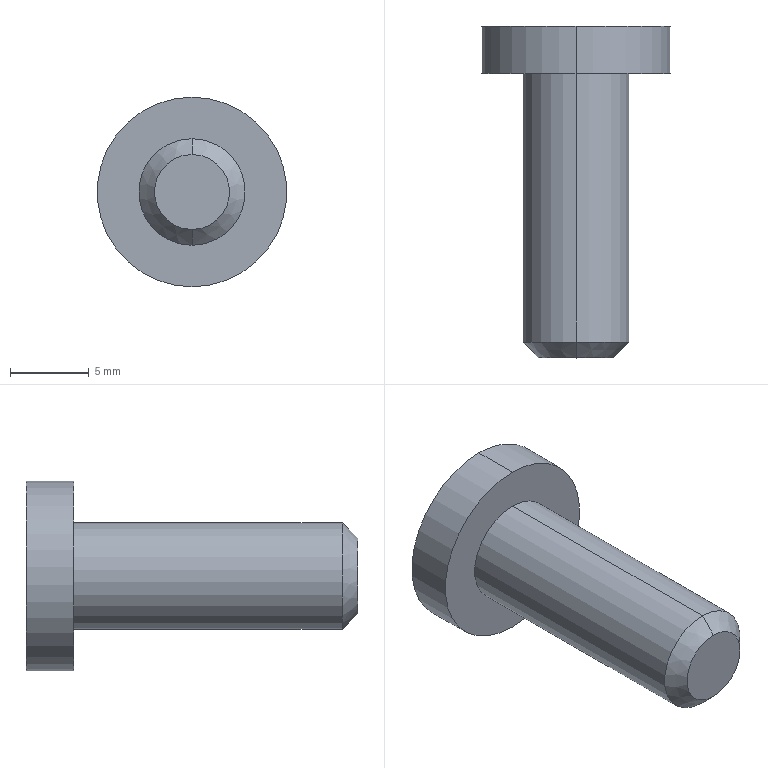Part | SolidWorks | features Chamfer 1, Revolution 1 | 1 solid | 9 faces | box 12 x 21 x 12 mm | volume 973.861 mm3 | cylinder 4 | plane 3 | cone 2 | commonest cylinder face diameters 6.75 x2 12 x2
STEP:
#1=CARTESIAN_POINT('',(-162.319,-426.852,-2.375));
#2=VERTEX_POINT('',#1);
#3=CARTESIAN_POINT('',(-162.319,-426.852,2.375));
#4=VERTEX_POINT('',#3);
#5=CARTESIAN_POINT('',(-162.319,-426.852,0.));
#6=DIRECTION('',(0.,-1.,0.));
#7=DIRECTION('',(0.,0.,1.));
#8=AXIS2_PLACEMENT_3D('',#5,#6,#7);
#9=CIRCLE('',#8,2.375);
#10=EDGE_CURVE('',#2,#4,#9,.T.);
#11=ORIENTED_EDGE('',*,*,#10,.F.);
#12=CARTESIAN_POINT('',(-162.319,-425.852,-3.375));
#13=VERTEX_POINT('',#12);
#14=CARTESIAN_POINT('',(-162.319,-425.852,-3.375));
#15=DIRECTION('',(0.,0.7071,-0.7071));
#16=VECTOR('',#15,1000.);
#17=LINE('',#14,#16);
#18=EDGE_CURVE('',#2,#13,#17,.T.);
#19=ORIENTED_EDGE('',*,*,#18,.T.);
#20=CARTESIAN_POINT('',(-162.319,-425.852,3.375));
#21=VERTEX_POINT('',#20);
#22=CARTESIAN_POINT('',(-162.319,-425.852,0.));
#23=DIRECTION('',(0.,1.,0.));
#24=DIRECTION('',(0.,0.,1.));
#25=AXIS2_PLACEMENT_3D('',#22,#23,#24);
#26=CIRCLE('',#25,3.375);
#27=EDGE_CURVE('',#21,#13,#26,.T.);
#28=ORIENTED_EDGE('',*,*,#27,.F.);
#29=CARTESIAN_POINT('',(-162.319,-425.852,3.375));
#30=DIRECTION('',(0.,0.7071,0.7071));
#31=VECTOR('',#30,1000.);
#32=LINE('',#29,#31);
#33=EDGE_CURVE('',#4,#21,#32,.T.);
#34=ORIENTED_EDGE('',*,*,#33,.F.);
#35=EDGE_LOOP('',(#11,#19,#28,#34));
#36=FACE_OUTER_BOUND('',#35,.T.);
#37=CARTESIAN_POINT('',(-162.319,-425.852,0.));
#38=DIRECTION('',(0.,1.,0.));
#39=DIRECTION('',(0.,0.,1.));
#40=AXIS2_PLACEMENT_3D('',#37,#38,#39);
#41=CONICAL_SURFACE('',#40,3.375,0.7854);
#42=ADVANCED_FACE('',(#36),#41,.T.);
#43=CARTESIAN_POINT('',(-162.319,-408.852,6.));
#44=VERTEX_POINT('',#43);
#45=CARTESIAN_POINT('',(-162.319,-408.852,-6.));
#46=VERTEX_POINT('',#45);
#47=CARTESIAN_POINT('',(-162.319,-408.852,0.));
#48=DIRECTION('',(0.,1.,0.));
#49=DIRECTION('',(0.,0.,1.));
#50=AXIS2_PLACEMENT_3D('',#47,#48,#49);
#51=CIRCLE('',#50,6.);
#52=EDGE_CURVE('',#44,#46,#51,.T.);
#53=ORIENTED_EDGE('',*,*,#52,.T.);
#54=CARTESIAN_POINT('',(-162.319,-405.852,-6.));
#55=VERTEX_POINT('',#54);
#56=CARTESIAN_POINT('',(-162.319,-405.852,-6.));
#57=DIRECTION('',(0.,1.,0.));
#58=VECTOR('',#57,1000.);
#59=LINE('',#56,#58);
#60=EDGE_CURVE('',#46,#55,#59,.T.);
#61=ORIENTED_EDGE('',*,*,#60,.T.);
#62=CARTESIAN_POINT('',(-162.319,-405.852,6.));
#63=VERTEX_POINT('',#62);
#64=CARTESIAN_POINT('',(-162.319,-405.852,0.));
#65=DIRECTION('',(0.,1.,0.));
#66=DIRECTION('',(0.,0.,1.));
#67=AXIS2_PLACEMENT_3D('',#64,#65,#66);
#68=CIRCLE('',#67,6.);
#69=EDGE_CURVE('',#63,#55,#68,.T.);
#70=ORIENTED_EDGE('',*,*,#69,.F.);
#71=CARTESIAN_POINT('',(-162.319,-405.852,6.));
#72=DIRECTION('',(0.,1.,0.));
#73=VECTOR('',#72,1000.);
#74=LINE('',#71,#73);
#75=EDGE_CURVE('',#44,#63,#74,.T.);
#76=ORIENTED_EDGE('',*,*,#75,.F.);
#77=EDGE_LOOP('',(#53,#61,#70,#76));
#78=FACE_OUTER_BOUND('',#77,.T.);
#79=CARTESIAN_POINT('',(-162.319,-405.852,0.));
#80=DIRECTION('',(0.,1.,0.));
#81=DIRECTION('',(0.,0.,1.));
#82=AXIS2_PLACEMENT_3D('',#79,#80,#81);
#83=CYLINDRICAL_SURFACE('',#82,6.);
#84=ADVANCED_FACE('',(#78),#83,.T.);
#85=ORIENTED_EDGE('',*,*,#27,.T.);
#86=CARTESIAN_POINT('',(-162.319,-408.852,-3.375));
#87=VERTEX_POINT('',#86);
#88=CARTESIAN_POINT('',(-162.319,-405.852,-3.375));
#89=DIRECTION('',(0.,1.,0.));
#90=VECTOR('',#89,1000.);
#91=LINE('',#88,#90);
#92=EDGE_CURVE('',#13,#87,#91,.T.);
#93=ORIENTED_EDGE('',*,*,#92,.T.);
#94=CARTESIAN_POINT('',(-162.319,-408.852,3.375));
#95=VERTEX_POINT('',#94);
#96=CARTESIAN_POINT('',(-162.319,-408.852,0.));
#97=DIRECTION('',(0.,1.,0.));
#98=DIRECTION('',(0.,0.,1.));
#99=AXIS2_PLACEMENT_3D('',#96,#97,#98);
#100=CIRCLE('',#99,3.375);
#101=EDGE_CURVE('',#95,#87,#100,.T.);
#102=ORIENTED_EDGE('',*,*,#101,.F.);
#103=CARTESIAN_POINT('',(-162.319,-405.852,3.375));
#104=DIRECTION('',(0.,1.,0.));
#105=VECTOR('',#104,1000.);
#106=LINE('',#103,#105);
#107=EDGE_CURVE('',#21,#95,#106,.T.);
#108=ORIENTED_EDGE('',*,*,#107,.F.);
#109=EDGE_LOOP('',(#85,#93,#102,#108));
#110=FACE_OUTER_BOUND('',#109,.T.);
#111=CARTESIAN_POINT('',(-162.319,-405.852,0.));
#112=DIRECTION('',(0.,1.,0.));
#113=DIRECTION('',(0.,0.,1.));
#114=AXIS2_PLACEMENT_3D('',#111,#112,#113);
#115=CYLINDRICAL_SURFACE('',#114,3.375);
#116=ADVANCED_FACE('',(#110),#115,.T.);
#117=ORIENTED_EDGE('',*,*,#69,.T.);
#118=CARTESIAN_POINT('',(-162.319,-405.852,0.));
#119=DIRECTION('',(0.,1.,0.));
#120=DIRECTION('',(0.,0.,1.));
#121=AXIS2_PLACEMENT_3D('',#118,#119,#120);
#122=CIRCLE('',#121,6.);
#123=EDGE_CURVE('',#55,#63,#122,.T.);
#124=ORIENTED_EDGE('',*,*,#123,.T.);
#125=EDGE_LOOP('',(#117,#124));
#126=FACE_OUTER_BOUND('',#125,.T.);
#127=CARTESIAN_POINT('',(-156.319,-405.852,0.));
#128=DIRECTION('',(0.,-1.,0.));
#129=DIRECTION('',(0.,0.,-1.));
#130=AXIS2_PLACEMENT_3D('',#127,#128,#129);
#131=PLANE('',#130);
#132=ADVANCED_FACE('',(#126),#131,.F.);
#133=CARTESIAN_POINT('',(-162.319,-426.852,0.));
#134=DIRECTION('',(0.,-1.,0.));
#135=DIRECTION('',(0.,0.,1.));
#136=AXIS2_PLACEMENT_3D('',#133,#134,#135);
#137=CIRCLE('',#136,2.375);
#138=EDGE_CURVE('',#4,#2,#137,.T.);
#139=ORIENTED_EDGE('',*,*,#138,.T.);
#140=ORIENTED_EDGE('',*,*,#10,.T.);
#141=EDGE_LOOP('',(#139,#140));
#142=FACE_OUTER_BOUND('',#141,.T.);
#143=CARTESIAN_POINT('',(-158.944,-426.852,0.));
#144=DIRECTION('',(0.,1.,0.));
#145=DIRECTION('',(0.,0.,1.));
#146=AXIS2_PLACEMENT_3D('',#143,#144,#145);
#147=PLANE('',#146);
#148=ADVANCED_FACE('',(#142),#147,.F.);
#149=ORIENTED_EDGE('',*,*,#92,.F.);
#150=CARTESIAN_POINT('',(-162.319,-425.852,0.));
#151=DIRECTION('',(0.,1.,0.));
#152=DIRECTION('',(0.,0.,1.));
#153=AXIS2_PLACEMENT_3D('',#150,#151,#152);
#154=CIRCLE('',#153,3.375);
#155=EDGE_CURVE('',#13,#21,#154,.T.);
#156=ORIENTED_EDGE('',*,*,#155,.T.);
#157=ORIENTED_EDGE('',*,*,#107,.T.);
#158=CARTESIAN_POINT('',(-162.319,-408.852,0.));
#159=DIRECTION('',(0.,1.,0.));
#160=DIRECTION('',(0.,0.,1.));
#161=AXIS2_PLACEMENT_3D('',#158,#159,#160);
#162=CIRCLE('',#161,3.375);
#163=EDGE_CURVE('',#87,#95,#162,.T.);
#164=ORIENTED_EDGE('',*,*,#163,.F.);
#165=EDGE_LOOP('',(#149,#156,#157,#164));
#166=FACE_OUTER_BOUND('',#165,.T.);
#167=CARTESIAN_POINT('',(-162.319,-405.852,0.));
#168=DIRECTION('',(0.,1.,0.));
#169=DIRECTION('',(0.,0.,1.));
#170=AXIS2_PLACEMENT_3D('',#167,#168,#169);
#171=CYLINDRICAL_SURFACE('',#170,3.375);
#172=ADVANCED_FACE('',(#166),#171,.T.);
#173=ORIENTED_EDGE('',*,*,#52,.F.);
#174=CARTESIAN_POINT('',(-162.319,-408.852,0.));
#175=DIRECTION('',(0.,1.,0.));
#176=DIRECTION('',(0.,0.,1.));
#177=AXIS2_PLACEMENT_3D('',#174,#175,#176);
#178=CIRCLE('',#177,6.);
#179=EDGE_CURVE('',#46,#44,#178,.T.);
#180=ORIENTED_EDGE('',*,*,#179,.F.);
#181=EDGE_LOOP('',(#173,#180));
#182=FACE_OUTER_BOUND('',#181,.T.);
#183=ORIENTED_EDGE('',*,*,#101,.T.);
#184=ORIENTED_EDGE('',*,*,#163,.T.);
#185=EDGE_LOOP('',(#183,#184));
#186=FACE_BOUND('',#185,.T.);
#187=CARTESIAN_POINT('',(-158.944,-408.852,0.));
#188=DIRECTION('',(0.,1.,0.));
#189=DIRECTION('',(0.,0.,1.));
#190=AXIS2_PLACEMENT_3D('',#187,#188,#189);
#191=PLANE('',#190);
#192=ADVANCED_FACE('',(#182,#186),#191,.F.);
#193=ORIENTED_EDGE('',*,*,#60,.F.);
#194=ORIENTED_EDGE('',*,*,#179,.T.);
#195=ORIENTED_EDGE('',*,*,#75,.T.);
#196=ORIENTED_EDGE('',*,*,#123,.F.);
#197=EDGE_LOOP('',(#193,#194,#195,#196));
#198=FACE_OUTER_BOUND('',#197,.T.);
#199=CARTESIAN_POINT('',(-162.319,-405.852,0.));
#200=DIRECTION('',(0.,1.,0.));
#201=DIRECTION('',(0.,0.,1.));
#202=AXIS2_PLACEMENT_3D('',#199,#200,#201);
#203=CYLINDRICAL_SURFACE('',#202,6.);
#204=ADVANCED_FACE('',(#198),#203,.T.);
#205=ORIENTED_EDGE('',*,*,#18,.F.);
#206=ORIENTED_EDGE('',*,*,#138,.F.);
#207=ORIENTED_EDGE('',*,*,#33,.T.);
#208=ORIENTED_EDGE('',*,*,#155,.F.);
#209=EDGE_LOOP('',(#205,#206,#207,#208));
#210=FACE_OUTER_BOUND('',#209,.T.);
#211=CARTESIAN_POINT('',(-162.319,-425.852,0.));
#212=DIRECTION('',(0.,1.,0.));
#213=DIRECTION('',(0.,0.,1.));
#214=AXIS2_PLACEMENT_3D('',#211,#212,#213);
#215=CONICAL_SURFACE('',#214,3.375,0.7854);
#216=ADVANCED_FACE('',(#210),#215,.T.);
#217=CLOSED_SHELL('',(#42,#84,#116,#132,#148,#172,#192,#204,#216));
#218=MANIFOLD_SOLID_BREP('',#217);
#219=CARTESIAN_POINT('',(0.,0.,0.));
#220=DIRECTION('',(0.,0.,1.));
#221=DIRECTION('',(1.,0.,0.));
#222=AXIS2_PLACEMENT_3D('',#219,#220,#221);
#223=(LENGTH_UNIT()NAMED_UNIT(*)SI_UNIT(.MILLI.,.METRE.));
#224=UNCERTAINTY_MEASURE_WITH_UNIT(LENGTH_MEASURE(0.00001),#223,'','');
#225=(NAMED_UNIT(*)PLANE_ANGLE_UNIT()SI_UNIT($,.RADIAN.));
#226=(NAMED_UNIT(*)SI_UNIT($,.STERADIAN.)SOLID_ANGLE_UNIT());
#227=(GEOMETRIC_REPRESENTATION_CONTEXT(3)GLOBAL_UNCERTAINTY_ASSIGNED_CONTEXT((#224))GLOBAL_UNIT_ASSIGNED_CONTEXT((#223,#225,#226))REPRESENTATION_CONTEXT('',''));
#228=ADVANCED_BREP_SHAPE_REPRESENTATION('',(#218,#222),#227);